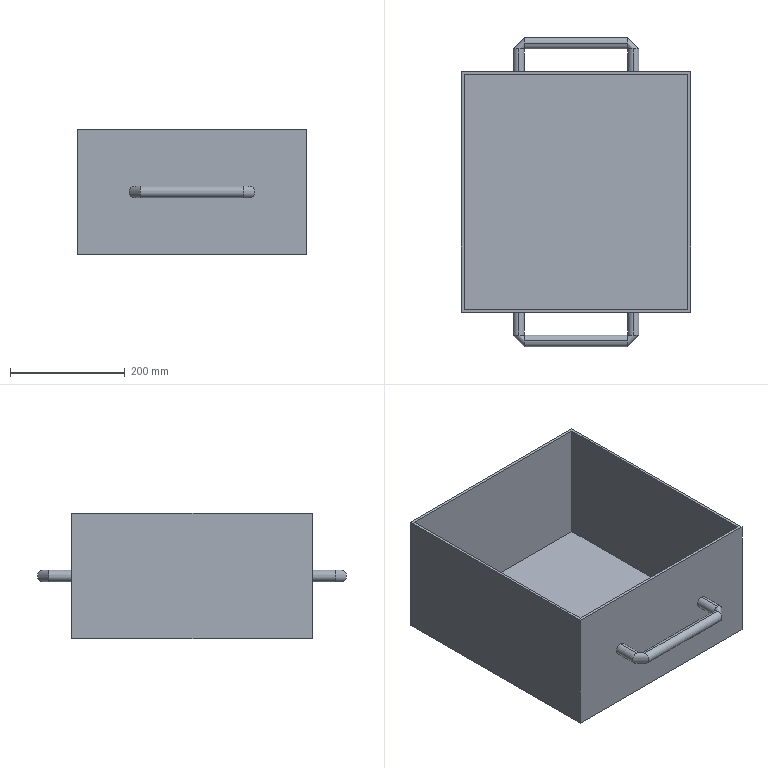Part | STEP file | Scrap collection box | 1 solid | 27 faces | box 400 x 540 x 220 mm | volume 2744863 mm3 | cylinder 12 | plane 11 | torus 4 | commonest cylinder face diameters 20 x12
STEP:
#1=CARTESIAN_POINT('',(100.,250.,-10.));
#2=VERTEX_POINT('',#1);
#3=CARTESIAN_POINT('',(100.,250.,10.));
#4=VERTEX_POINT('',#3);
#5=CARTESIAN_POINT('',(100.,250.,0.));
#6=DIRECTION('',(0.,-1.,0.));
#7=DIRECTION('',(0.,0.,-1.));
#8=AXIS2_PLACEMENT_3D('',#5,#6,#7);
#9=CIRCLE('',#8,10.);
#10=EDGE_CURVE('',#2,#4,#9,.T.);
#11=ORIENTED_EDGE('',*,*,#10,.T.);
#12=CARTESIAN_POINT('',(100.,210.,10.));
#13=VERTEX_POINT('',#12);
#14=CARTESIAN_POINT('',(100.,250.,10.));
#15=DIRECTION('',(0.,-1.,0.));
#16=VECTOR('',#15,1000.);
#17=LINE('',#14,#16);
#18=EDGE_CURVE('',#4,#13,#17,.T.);
#19=ORIENTED_EDGE('',*,*,#18,.T.);
#20=CARTESIAN_POINT('',(100.,210.,-10.));
#21=VERTEX_POINT('',#20);
#22=CARTESIAN_POINT('',(100.,210.,0.));
#23=DIRECTION('',(0.,-1.,0.));
#24=DIRECTION('',(0.,0.,-1.));
#25=AXIS2_PLACEMENT_3D('',#22,#23,#24);
#26=CIRCLE('',#25,10.);
#27=EDGE_CURVE('',#21,#13,#26,.T.);
#28=ORIENTED_EDGE('',*,*,#27,.F.);
#29=CARTESIAN_POINT('',(100.,250.,-10.));
#30=DIRECTION('',(0.,-1.,0.));
#31=VECTOR('',#30,1000.);
#32=LINE('',#29,#31);
#33=EDGE_CURVE('',#2,#21,#32,.T.);
#34=ORIENTED_EDGE('',*,*,#33,.F.);
#35=EDGE_LOOP('',(#11,#19,#28,#34));
#36=FACE_OUTER_BOUND('',#35,.T.);
#37=CARTESIAN_POINT('',(100.,250.,0.));
#38=DIRECTION('',(0.,-1.,0.));
#39=DIRECTION('',(0.,0.,-1.));
#40=AXIS2_PLACEMENT_3D('',#37,#38,#39);
#41=CYLINDRICAL_SURFACE('',#40,10.);
#42=ADVANCED_FACE('',(#36),#41,.T.);
#43=CARTESIAN_POINT('',(-90.,260.,-10.));
#44=VERTEX_POINT('',#43);
#45=CARTESIAN_POINT('',(-90.,260.,10.));
#46=VERTEX_POINT('',#45);
#47=CARTESIAN_POINT('',(-90.,260.,0.));
#48=DIRECTION('',(1.,0.,0.));
#49=DIRECTION('',(0.,0.,-1.));
#50=AXIS2_PLACEMENT_3D('',#47,#48,#49);
#51=CIRCLE('',#50,10.);
#52=EDGE_CURVE('',#44,#46,#51,.T.);
#53=ORIENTED_EDGE('',*,*,#52,.T.);
#54=CARTESIAN_POINT('',(90.,260.,10.));
#55=VERTEX_POINT('',#54);
#56=CARTESIAN_POINT('',(-90.,260.,10.));
#57=DIRECTION('',(1.,0.,0.));
#58=VECTOR('',#57,1000.);
#59=LINE('',#56,#58);
#60=EDGE_CURVE('',#46,#55,#59,.T.);
#61=ORIENTED_EDGE('',*,*,#60,.T.);
#62=CARTESIAN_POINT('',(90.,260.,-10.));
#63=VERTEX_POINT('',#62);
#64=CARTESIAN_POINT('',(90.,260.,0.));
#65=DIRECTION('',(1.,0.,0.));
#66=DIRECTION('',(0.,0.,-1.));
#67=AXIS2_PLACEMENT_3D('',#64,#65,#66);
#68=CIRCLE('',#67,10.);
#69=EDGE_CURVE('',#63,#55,#68,.T.);
#70=ORIENTED_EDGE('',*,*,#69,.F.);
#71=CARTESIAN_POINT('',(-90.,260.,-10.));
#72=DIRECTION('',(1.,0.,0.));
#73=VECTOR('',#72,1000.);
#74=LINE('',#71,#73);
#75=EDGE_CURVE('',#44,#63,#74,.T.);
#76=ORIENTED_EDGE('',*,*,#75,.F.);
#77=EDGE_LOOP('',(#53,#61,#70,#76));
#78=FACE_OUTER_BOUND('',#77,.T.);
#79=CARTESIAN_POINT('',(-90.,260.,0.));
#80=DIRECTION('',(1.,0.,0.));
#81=DIRECTION('',(0.,0.,-1.));
#82=AXIS2_PLACEMENT_3D('',#79,#80,#81);
#83=CYLINDRICAL_SURFACE('',#82,10.);
#84=ADVANCED_FACE('',(#78),#83,.T.);
#85=CARTESIAN_POINT('',(-100.,210.,10.));
#86=VERTEX_POINT('',#85);
#87=CARTESIAN_POINT('',(-100.,210.,-10.));
#88=VERTEX_POINT('',#87);
#89=CARTESIAN_POINT('',(-100.,210.,0.));
#90=DIRECTION('',(0.,1.,0.));
#91=DIRECTION('',(0.,0.,-1.));
#92=AXIS2_PLACEMENT_3D('',#89,#90,#91);
#93=CIRCLE('',#92,10.);
#94=EDGE_CURVE('',#86,#88,#93,.T.);
#95=ORIENTED_EDGE('',*,*,#94,.T.);
#96=CARTESIAN_POINT('',(-100.,250.,-10.));
#97=VERTEX_POINT('',#96);
#98=CARTESIAN_POINT('',(-100.,210.,-10.));
#99=DIRECTION('',(0.,1.,0.));
#100=VECTOR('',#99,1000.);
#101=LINE('',#98,#100);
#102=EDGE_CURVE('',#88,#97,#101,.T.);
#103=ORIENTED_EDGE('',*,*,#102,.T.);
#104=CARTESIAN_POINT('',(-90.,250.,0.));
#105=VERTEX_POINT('',#104);
#106=CARTESIAN_POINT('',(-100.,250.,0.));
#107=DIRECTION('',(0.,1.,0.));
#108=DIRECTION('',(0.,0.,-1.));
#109=AXIS2_PLACEMENT_3D('',#106,#107,#108);
#110=CIRCLE('',#109,10.);
#111=EDGE_CURVE('',#105,#97,#110,.T.);
#112=ORIENTED_EDGE('',*,*,#111,.F.);
#113=CARTESIAN_POINT('',(-100.,250.,10.));
#114=VERTEX_POINT('',#113);
#115=CARTESIAN_POINT('',(-100.,250.,0.));
#116=DIRECTION('',(0.,1.,0.));
#117=DIRECTION('',(0.,0.,-1.));
#118=AXIS2_PLACEMENT_3D('',#115,#116,#117);
#119=CIRCLE('',#118,10.);
#120=EDGE_CURVE('',#114,#105,#119,.T.);
#121=ORIENTED_EDGE('',*,*,#120,.F.);
#122=CARTESIAN_POINT('',(-100.,210.,10.));
#123=DIRECTION('',(0.,1.,0.));
#124=VECTOR('',#123,1000.);
#125=LINE('',#122,#124);
#126=EDGE_CURVE('',#86,#114,#125,.T.);
#127=ORIENTED_EDGE('',*,*,#126,.F.);
#128=EDGE_LOOP('',(#95,#103,#112,#121,#127));
#129=FACE_OUTER_BOUND('',#128,.T.);
#130=CARTESIAN_POINT('',(-100.,210.,0.));
#131=DIRECTION('',(0.,1.,0.));
#132=DIRECTION('',(0.,0.,1.));
#133=AXIS2_PLACEMENT_3D('',#130,#131,#132);
#134=CYLINDRICAL_SURFACE('',#133,10.);
#135=ADVANCED_FACE('',(#129),#134,.T.);
#136=CARTESIAN_POINT('',(100.,-250.,10.));
#137=VERTEX_POINT('',#136);
#138=CARTESIAN_POINT('',(100.,-250.,-10.));
#139=VERTEX_POINT('',#138);
#140=CARTESIAN_POINT('',(100.,-250.,0.));
#141=DIRECTION('',(0.,1.,0.));
#142=DIRECTION('',(0.,0.,-1.));
#143=AXIS2_PLACEMENT_3D('',#140,#141,#142);
#144=CIRCLE('',#143,10.);
#145=EDGE_CURVE('',#137,#139,#144,.T.);
#146=ORIENTED_EDGE('',*,*,#145,.T.);
#147=CARTESIAN_POINT('',(100.,-210.,-10.));
#148=VERTEX_POINT('',#147);
#149=CARTESIAN_POINT('',(100.,-250.,-10.));
#150=DIRECTION('',(0.,1.,0.));
#151=VECTOR('',#150,1000.);
#152=LINE('',#149,#151);
#153=EDGE_CURVE('',#139,#148,#152,.T.);
#154=ORIENTED_EDGE('',*,*,#153,.T.);
#155=CARTESIAN_POINT('',(100.,-210.,10.));
#156=VERTEX_POINT('',#155);
#157=CARTESIAN_POINT('',(100.,-210.,0.));
#158=DIRECTION('',(0.,1.,0.));
#159=DIRECTION('',(0.,0.,-1.));
#160=AXIS2_PLACEMENT_3D('',#157,#158,#159);
#161=CIRCLE('',#160,10.);
#162=EDGE_CURVE('',#156,#148,#161,.T.);
#163=ORIENTED_EDGE('',*,*,#162,.F.);
#164=CARTESIAN_POINT('',(100.,-250.,10.));
#165=DIRECTION('',(0.,1.,0.));
#166=VECTOR('',#165,1000.);
#167=LINE('',#164,#166);
#168=EDGE_CURVE('',#137,#156,#167,.T.);
#169=ORIENTED_EDGE('',*,*,#168,.F.);
#170=EDGE_LOOP('',(#146,#154,#163,#169));
#171=FACE_OUTER_BOUND('',#170,.T.);
#172=CARTESIAN_POINT('',(100.,-250.,0.));
#173=DIRECTION('',(0.,1.,0.));
#174=DIRECTION('',(0.,0.,1.));
#175=AXIS2_PLACEMENT_3D('',#172,#173,#174);
#176=CYLINDRICAL_SURFACE('',#175,10.);
#177=ADVANCED_FACE('',(#171),#176,.T.);
#178=CARTESIAN_POINT('',(-90.,-250.,0.));
#179=VERTEX_POINT('',#178);
#180=CARTESIAN_POINT('',(-90.,-260.,10.));
#181=VERTEX_POINT('',#180);
#182=CARTESIAN_POINT('',(-90.,-260.,0.));
#183=DIRECTION('',(1.,0.,0.));
#184=DIRECTION('',(0.,0.,-1.));
#185=AXIS2_PLACEMENT_3D('',#182,#183,#184);
#186=CIRCLE('',#185,10.);
#187=EDGE_CURVE('',#179,#181,#186,.T.);
#188=ORIENTED_EDGE('',*,*,#187,.T.);
#189=CARTESIAN_POINT('',(90.,-260.,10.));
#190=VERTEX_POINT('',#189);
#191=CARTESIAN_POINT('',(-90.,-260.,10.));
#192=DIRECTION('',(1.,0.,0.));
#193=VECTOR('',#192,1000.);
#194=LINE('',#191,#193);
#195=EDGE_CURVE('',#181,#190,#194,.T.);
#196=ORIENTED_EDGE('',*,*,#195,.T.);
#197=CARTESIAN_POINT('',(90.,-250.,0.));
#198=VERTEX_POINT('',#197);
#199=CARTESIAN_POINT('',(90.,-260.,0.));
#200=DIRECTION('',(1.,0.,0.));
#201=DIRECTION('',(0.,0.,-1.));
#202=AXIS2_PLACEMENT_3D('',#199,#200,#201);
#203=CIRCLE('',#202,10.);
#204=EDGE_CURVE('',#198,#190,#203,.T.);
#205=ORIENTED_EDGE('',*,*,#204,.F.);
#206=CARTESIAN_POINT('',(90.,-260.,-10.));
#207=VERTEX_POINT('',#206);
#208=CARTESIAN_POINT('',(90.,-260.,0.));
#209=DIRECTION('',(1.,0.,0.));
#210=DIRECTION('',(0.,0.,-1.));
#211=AXIS2_PLACEMENT_3D('',#208,#209,#210);
#212=CIRCLE('',#211,10.);
#213=EDGE_CURVE('',#207,#198,#212,.T.);
#214=ORIENTED_EDGE('',*,*,#213,.F.);
#215=CARTESIAN_POINT('',(-90.,-260.,-10.));
#216=VERTEX_POINT('',#215);
#217=CARTESIAN_POINT('',(-90.,-260.,-10.));
#218=DIRECTION('',(1.,0.,0.));
#219=VECTOR('',#218,1000.);
#220=LINE('',#217,#219);
#221=EDGE_CURVE('',#216,#207,#220,.T.);
#222=ORIENTED_EDGE('',*,*,#221,.F.);
#223=CARTESIAN_POINT('',(-90.,-260.,0.));
#224=DIRECTION('',(1.,0.,0.));
#225=DIRECTION('',(0.,0.,-1.));
#226=AXIS2_PLACEMENT_3D('',#223,#224,#225);
#227=CIRCLE('',#226,10.);
#228=EDGE_CURVE('',#216,#179,#227,.T.);
#229=ORIENTED_EDGE('',*,*,#228,.T.);
#230=EDGE_LOOP('',(#188,#196,#205,#214,#222,#229));
#231=FACE_OUTER_BOUND('',#230,.T.);
#232=CARTESIAN_POINT('',(-90.,-260.,0.));
#233=DIRECTION('',(1.,0.,0.));
#234=DIRECTION('',(0.,0.,-1.));
#235=AXIS2_PLACEMENT_3D('',#232,#233,#234);
#236=CYLINDRICAL_SURFACE('',#235,10.);
#237=ADVANCED_FACE('',(#231),#236,.T.);
#238=CARTESIAN_POINT('',(-100.,-210.,-10.));
#239=VERTEX_POINT('',#238);
#240=CARTESIAN_POINT('',(-100.,-210.,10.));
#241=VERTEX_POINT('',#240);
#242=CARTESIAN_POINT('',(-100.,-210.,0.));
#243=DIRECTION('',(0.,-1.,0.));
#244=DIRECTION('',(0.,0.,-1.));
#245=AXIS2_PLACEMENT_3D('',#242,#243,#244);
#246=CIRCLE('',#245,10.);
#247=EDGE_CURVE('',#239,#241,#246,.T.);
#248=ORIENTED_EDGE('',*,*,#247,.T.);
#249=CARTESIAN_POINT('',(-100.,-250.,10.));
#250=VERTEX_POINT('',#249);
#251=CARTESIAN_POINT('',(-100.,-210.,10.));
#252=DIRECTION('',(0.,-1.,0.));
#253=VECTOR('',#252,1000.);
#254=LINE('',#251,#253);
#255=EDGE_CURVE('',#241,#250,#254,.T.);
#256=ORIENTED_EDGE('',*,*,#255,.T.);
#257=CARTESIAN_POINT('',(-100.,-250.,0.));
#258=DIRECTION('',(0.,-1.,0.));
#259=DIRECTION('',(0.,0.,-1.));
#260=AXIS2_PLACEMENT_3D('',#257,#258,#259);
#261=CIRCLE('',#260,10.);
#262=EDGE_CURVE('',#179,#250,#261,.T.);
#263=ORIENTED_EDGE('',*,*,#262,.F.);
#264=CARTESIAN_POINT('',(-100.,-250.,-10.));
#265=VERTEX_POINT('',#264);
#266=CARTESIAN_POINT('',(-100.,-250.,0.));
#267=DIRECTION('',(0.,-1.,0.));
#268=DIRECTION('',(0.,0.,-1.));
#269=AXIS2_PLACEMENT_3D('',#266,#267,#268);
#270=CIRCLE('',#269,10.);
#271=EDGE_CURVE('',#265,#179,#270,.T.);
#272=ORIENTED_EDGE('',*,*,#271,.F.);
#273=CARTESIAN_POINT('',(-100.,-210.,-10.));
#274=DIRECTION('',(0.,-1.,0.));
#275=VECTOR('',#274,1000.);
#276=LINE('',#273,#275);
#277=EDGE_CURVE('',#239,#265,#276,.T.);
#278=ORIENTED_EDGE('',*,*,#277,.F.);
#279=EDGE_LOOP('',(#248,#256,#263,#272,#278));
#280=FACE_OUTER_BOUND('',#279,.T.);
#281=CARTESIAN_POINT('',(-100.,-210.,0.));
#282=DIRECTION('',(0.,-1.,0.));
#283=DIRECTION('',(0.,0.,-1.));
#284=AXIS2_PLACEMENT_3D('',#281,#282,#283);
#285=CYLINDRICAL_SURFACE('',#284,10.);
#286=ADVANCED_FACE('',(#280),#285,.T.);
#287=CARTESIAN_POINT('',(200.,-210.,-110.));
#288=VERTEX_POINT('',#287);
#289=CARTESIAN_POINT('',(200.,210.,-110.));
#290=VERTEX_POINT('',#289);
#291=CARTESIAN_POINT('',(200.,210.,-110.));
#292=DIRECTION('',(0.,1.,0.));
#293=VECTOR('',#292,1000.);
#294=LINE('',#291,#293);
#295=EDGE_CURVE('',#288,#290,#294,.T.);
#296=ORIENTED_EDGE('',*,*,#295,.T.);
#297=CARTESIAN_POINT('',(200.,210.,110.));
#298=VERTEX_POINT('',#297);
#299=CARTESIAN_POINT('',(200.,210.,110.));
#300=DIRECTION('',(0.,0.,-1.));
#301=VECTOR('',#300,1000.);
#302=LINE('',#299,#301);
#303=EDGE_CURVE('',#298,#290,#302,.T.);
#304=ORIENTED_EDGE('',*,*,#303,.F.);
#305=CARTESIAN_POINT('',(200.,-210.,110.));
#306=VERTEX_POINT('',#305);
#307=CARTESIAN_POINT('',(200.,210.,110.));
#308=DIRECTION('',(0.,1.,0.));
#309=VECTOR('',#308,1000.);
#310=LINE('',#307,#309);
#311=EDGE_CURVE('',#306,#298,#310,.T.);
#312=ORIENTED_EDGE('',*,*,#311,.F.);
#313=CARTESIAN_POINT('',(200.,-210.,110.));
#314=DIRECTION('',(0.,0.,-1.));
#315=VECTOR('',#314,1000.);
#316=LINE('',#313,#315);
#317=EDGE_CURVE('',#306,#288,#316,.T.);
#318=ORIENTED_EDGE('',*,*,#317,.T.);
#319=EDGE_LOOP('',(#296,#304,#312,#318));
#320=FACE_OUTER_BOUND('',#319,.T.);
#321=CARTESIAN_POINT('',(200.,210.,110.));
#322=DIRECTION('',(-1.,0.,0.));
#323=DIRECTION('',(0.,-1.,0.));
#324=AXIS2_PLACEMENT_3D('',#321,#322,#323);
#325=PLANE('',#324);
#326=ADVANCED_FACE('',(#320),#325,.F.);
#327=ORIENTED_EDGE('',*,*,#94,.F.);
#328=CARTESIAN_POINT('',(-100.,210.,0.));
#329=DIRECTION('',(0.,1.,0.));
#330=DIRECTION('',(0.,0.,-1.));
#331=AXIS2_PLACEMENT_3D('',#328,#329,#330);
#332=CIRCLE('',#331,10.);
#333=EDGE_CURVE('',#88,#86,#332,.T.);
#334=ORIENTED_EDGE('',*,*,#333,.F.);
#335=EDGE_LOOP('',(#327,#334));
#336=FACE_BOUND('',#335,.T.);
#337=ORIENTED_EDGE('',*,*,#27,.T.);
#338=CARTESIAN_POINT('',(100.,210.,0.));
#339=DIRECTION('',(0.,-1.,0.));
#340=DIRECTION('',(0.,0.,-1.));
#341=AXIS2_PLACEMENT_3D('',#338,#339,#340);
#342=CIRCLE('',#341,10.);
#343=EDGE_CURVE('',#13,#21,#342,.T.);
#344=ORIENTED_EDGE('',*,*,#343,.T.);
#345=EDGE_LOOP('',(#337,#344));
#346=FACE_BOUND('',#345,.T.);
#347=CARTESIAN_POINT('',(-200.,210.,-110.));
#348=VERTEX_POINT('',#347);
#349=CARTESIAN_POINT('',(-200.,210.,-110.));
#350=DIRECTION('',(-1.,0.,0.));
#351=VECTOR('',#350,1000.);
#352=LINE('',#349,#351);
#353=EDGE_CURVE('',#290,#348,#352,.T.);
#354=ORIENTED_EDGE('',*,*,#353,.T.);
#355=CARTESIAN_POINT('',(-200.,210.,110.));
#356=VERTEX_POINT('',#355);
#357=CARTESIAN_POINT('',(-200.,210.,110.));
#358=DIRECTION('',(0.,0.,-1.));
#359=VECTOR('',#358,1000.);
#360=LINE('',#357,#359);
#361=EDGE_CURVE('',#356,#348,#360,.T.);
#362=ORIENTED_EDGE('',*,*,#361,.F.);
#363=CARTESIAN_POINT('',(-200.,210.,110.));
#364=DIRECTION('',(-1.,0.,0.));
#365=VECTOR('',#364,1000.);
#366=LINE('',#363,#365);
#367=EDGE_CURVE('',#298,#356,#366,.T.);
#368=ORIENTED_EDGE('',*,*,#367,.F.);
#369=ORIENTED_EDGE('',*,*,#303,.T.);
#370=EDGE_LOOP('',(#354,#362,#368,#369));
#371=FACE_OUTER_BOUND('',#370,.T.);
#372=CARTESIAN_POINT('',(-200.,210.,110.));
#373=DIRECTION('',(0.,-1.,0.));
#374=DIRECTION('',(0.,0.,-1.));
#375=AXIS2_PLACEMENT_3D('',#372,#373,#374);
#376=PLANE('',#375);
#377=ADVANCED_FACE('',(#336,#346,#371),#376,.F.);
#378=CARTESIAN_POINT('',(-200.,-210.,-110.));
#379=VERTEX_POINT('',#378);
#380=CARTESIAN_POINT('',(-200.,210.,-110.));
#381=DIRECTION('',(0.,-1.,0.));
#382=VECTOR('',#381,1000.);
#383=LINE('',#380,#382);
#384=EDGE_CURVE('',#348,#379,#383,.T.);
#385=ORIENTED_EDGE('',*,*,#384,.T.);
#386=CARTESIAN_POINT('',(-200.,-210.,110.));
#387=VERTEX_POINT('',#386);
#388=CARTESIAN_POINT('',(-200.,-210.,110.));
#389=DIRECTION('',(0.,0.,-1.));
#390=VECTOR('',#389,1000.);
#391=LINE('',#388,#390);
#392=EDGE_CURVE('',#387,#379,#391,.T.);
#393=ORIENTED_EDGE('',*,*,#392,.F.);
#394=CARTESIAN_POINT('',(-200.,210.,110.));
#395=DIRECTION('',(0.,-1.,0.));
#396=VECTOR('',#395,1000.);
#397=LINE('',#394,#396);
#398=EDGE_CURVE('',#356,#387,#397,.T.);
#399=ORIENTED_EDGE('',*,*,#398,.F.);
#400=ORIENTED_EDGE('',*,*,#361,.T.);
#401=EDGE_LOOP('',(#385,#393,#399,#400));
#402=FACE_OUTER_BOUND('',#401,.T.);
#403=CARTESIAN_POINT('',(-200.,210.,110.));
#404=DIRECTION('',(1.,0.,0.));
#405=DIRECTION('',(0.,1.,0.));
#406=AXIS2_PLACEMENT_3D('',#403,#404,#405);
#407=PLANE('',#406);
#408=ADVANCED_FACE('',(#402),#407,.F.);
#409=ORIENTED_EDGE('',*,*,#247,.F.);
#410=CARTESIAN_POINT('',(-100.,-210.,0.));
#411=DIRECTION('',(0.,-1.,0.));
#412=DIRECTION('',(0.,0.,-1.));
#413=AXIS2_PLACEMENT_3D('',#410,#411,#412);
#414=CIRCLE('',#413,10.);
#415=EDGE_CURVE('',#241,#239,#414,.T.);
#416=ORIENTED_EDGE('',*,*,#415,.F.);
#417=EDGE_LOOP('',(#409,#416));
#418=FACE_BOUND('',#417,.T.);
#419=ORIENTED_EDGE('',*,*,#162,.T.);
#420=CARTESIAN_POINT('',(100.,-210.,0.));
#421=DIRECTION('',(0.,1.,0.));
#422=DIRECTION('',(0.,0.,-1.));
#423=AXIS2_PLACEMENT_3D('',#420,#421,#422);
#424=CIRCLE('',#423,10.);
#425=EDGE_CURVE('',#148,#156,#424,.T.);
#426=ORIENTED_EDGE('',*,*,#425,.T.);
#427=EDGE_LOOP('',(#419,#426));
#428=FACE_BOUND('',#427,.T.);
#429=CARTESIAN_POINT('',(-200.,-210.,-110.));
#430=DIRECTION('',(1.,0.,0.));
#431=VECTOR('',#430,1000.);
#432=LINE('',#429,#431);
#433=EDGE_CURVE('',#379,#288,#432,.T.);
#434=ORIENTED_EDGE('',*,*,#433,.T.);
#435=ORIENTED_EDGE('',*,*,#317,.F.);
#436=CARTESIAN_POINT('',(-200.,-210.,110.));
#437=DIRECTION('',(1.,0.,0.));
#438=VECTOR('',#437,1000.);
#439=LINE('',#436,#438);
#440=EDGE_CURVE('',#387,#306,#439,.T.);
#441=ORIENTED_EDGE('',*,*,#440,.F.);
#442=ORIENTED_EDGE('',*,*,#392,.T.);
#443=EDGE_LOOP('',(#434,#435,#441,#442));
#444=FACE_OUTER_BOUND('',#443,.T.);
#445=CARTESIAN_POINT('',(-200.,-210.,110.));
#446=DIRECTION('',(0.,1.,0.));
#447=DIRECTION('',(0.,0.,1.));
#448=AXIS2_PLACEMENT_3D('',#445,#446,#447);
#449=PLANE('',#448);
#450=ADVANCED_FACE('',(#418,#428,#444),#449,.F.);
#451=CARTESIAN_POINT('',(195.,-205.,110.));
#452=VERTEX_POINT('',#451);
#453=CARTESIAN_POINT('',(195.,205.,110.));
#454=VERTEX_POINT('',#453);
#455=CARTESIAN_POINT('',(195.,210.,110.));
#456=DIRECTION('',(0.,1.,0.));
#457=VECTOR('',#456,1000.);
#458=LINE('',#455,#457);
#459=EDGE_CURVE('',#452,#454,#458,.T.);
#460=ORIENTED_EDGE('',*,*,#459,.F.);
#461=CARTESIAN_POINT('',(-195.,-205.,110.));
#462=VERTEX_POINT('',#461);
#463=CARTESIAN_POINT('',(-200.,-205.,110.));
#464=DIRECTION('',(1.,0.,0.));
#465=VECTOR('',#464,1000.);
#466=LINE('',#463,#465);
#467=EDGE_CURVE('',#462,#452,#466,.T.);
#468=ORIENTED_EDGE('',*,*,#467,.F.);
#469=CARTESIAN_POINT('',(-195.,205.,110.));
#470=VERTEX_POINT('',#469);
#471=CARTESIAN_POINT('',(-195.,210.,110.));
#472=DIRECTION('',(0.,-1.,0.));
#473=VECTOR('',#472,1000.);
#474=LINE('',#471,#473);
#475=EDGE_CURVE('',#470,#462,#474,.T.);
#476=ORIENTED_EDGE('',*,*,#475,.F.);
#477=CARTESIAN_POINT('',(-200.,205.,110.));
#478=DIRECTION('',(-1.,0.,0.));
#479=VECTOR('',#478,1000.);
#480=LINE('',#477,#479);
#481=EDGE_CURVE('',#454,#470,#480,.T.);
#482=ORIENTED_EDGE('',*,*,#481,.F.);
#483=EDGE_LOOP('',(#460,#468,#476,#482));
#484=FACE_BOUND('',#483,.T.);
#485=ORIENTED_EDGE('',*,*,#311,.T.);
#486=ORIENTED_EDGE('',*,*,#367,.T.);
#487=ORIENTED_EDGE('',*,*,#398,.T.);
#488=ORIENTED_EDGE('',*,*,#440,.T.);
#489=EDGE_LOOP('',(#485,#486,#487,#488));
#490=FACE_OUTER_BOUND('',#489,.T.);
#491=CARTESIAN_POINT('',(0.,0.,110.));
#492=DIRECTION('',(0.,0.,1.));
#493=DIRECTION('',(1.,0.,0.));
#494=AXIS2_PLACEMENT_3D('',#491,#492,#493);
#495=PLANE('',#494);
#496=ADVANCED_FACE('',(#484,#490),#495,.T.);
#497=ORIENTED_EDGE('',*,*,#295,.F.);
#498=ORIENTED_EDGE('',*,*,#433,.F.);
#499=ORIENTED_EDGE('',*,*,#384,.F.);
#500=ORIENTED_EDGE('',*,*,#353,.F.);
#501=EDGE_LOOP('',(#497,#498,#499,#500));
#502=FACE_OUTER_BOUND('',#501,.T.);
#503=CARTESIAN_POINT('',(0.,0.,-110.));
#504=DIRECTION('',(0.,0.,1.));
#505=DIRECTION('',(1.,0.,0.));
#506=AXIS2_PLACEMENT_3D('',#503,#504,#505);
#507=PLANE('',#506);
#508=ADVANCED_FACE('',(#502),#507,.F.);
#509=CARTESIAN_POINT('',(195.,-205.,-105.));
#510=VERTEX_POINT('',#509);
#511=CARTESIAN_POINT('',(195.,205.,-105.));
#512=VERTEX_POINT('',#511);
#513=CARTESIAN_POINT('',(195.,210.,-105.));
#514=DIRECTION('',(0.,1.,0.));
#515=VECTOR('',#514,1000.);
#516=LINE('',#513,#515);
#517=EDGE_CURVE('',#510,#512,#516,.T.);
#518=ORIENTED_EDGE('',*,*,#517,.F.);
#519=CARTESIAN_POINT('',(195.,-205.,110.));
#520=DIRECTION('',(0.,0.,-1.));
#521=VECTOR('',#520,1000.);
#522=LINE('',#519,#521);
#523=EDGE_CURVE('',#452,#510,#522,.T.);
#524=ORIENTED_EDGE('',*,*,#523,.F.);
#525=ORIENTED_EDGE('',*,*,#459,.T.);
#526=CARTESIAN_POINT('',(195.,205.,110.));
#527=DIRECTION('',(0.,0.,-1.));
#528=VECTOR('',#527,1000.);
#529=LINE('',#526,#528);
#530=EDGE_CURVE('',#454,#512,#529,.T.);
#531=ORIENTED_EDGE('',*,*,#530,.T.);
#532=EDGE_LOOP('',(#518,#524,#525,#531));
#533=FACE_OUTER_BOUND('',#532,.T.);
#534=CARTESIAN_POINT('',(195.,210.,110.));
#535=DIRECTION('',(-1.,0.,0.));
#536=DIRECTION('',(0.,-1.,0.));
#537=AXIS2_PLACEMENT_3D('',#534,#535,#536);
#538=PLANE('',#537);
#539=ADVANCED_FACE('',(#533),#538,.T.);
#540=CARTESIAN_POINT('',(-195.,205.,-105.));
#541=VERTEX_POINT('',#540);
#542=CARTESIAN_POINT('',(-200.,205.,-105.));
#543=DIRECTION('',(-1.,0.,0.));
#544=VECTOR('',#543,1000.);
#545=LINE('',#542,#544);
#546=EDGE_CURVE('',#512,#541,#545,.T.);
#547=ORIENTED_EDGE('',*,*,#546,.F.);
#548=ORIENTED_EDGE('',*,*,#530,.F.);
#549=ORIENTED_EDGE('',*,*,#481,.T.);
#550=CARTESIAN_POINT('',(-195.,205.,110.));
#551=DIRECTION('',(0.,0.,-1.));
#552=VECTOR('',#551,1000.);
#553=LINE('',#550,#552);
#554=EDGE_CURVE('',#470,#541,#553,.T.);
#555=ORIENTED_EDGE('',*,*,#554,.T.);
#556=EDGE_LOOP('',(#547,#548,#549,#555));
#557=FACE_OUTER_BOUND('',#556,.T.);
#558=CARTESIAN_POINT('',(-200.,205.,110.));
#559=DIRECTION('',(0.,-1.,0.));
#560=DIRECTION('',(0.,0.,-1.));
#561=AXIS2_PLACEMENT_3D('',#558,#559,#560);
#562=PLANE('',#561);
#563=ADVANCED_FACE('',(#557),#562,.T.);
#564=CARTESIAN_POINT('',(-195.,-205.,-105.));
#565=VERTEX_POINT('',#564);
#566=CARTESIAN_POINT('',(-195.,210.,-105.));
#567=DIRECTION('',(0.,-1.,0.));
#568=VECTOR('',#567,1000.);
#569=LINE('',#566,#568);
#570=EDGE_CURVE('',#541,#565,#569,.T.);
#571=ORIENTED_EDGE('',*,*,#570,.F.);
#572=ORIENTED_EDGE('',*,*,#554,.F.);
#573=ORIENTED_EDGE('',*,*,#475,.T.);
#574=CARTESIAN_POINT('',(-195.,-205.,110.));
#575=DIRECTION('',(0.,0.,-1.));
#576=VECTOR('',#575,1000.);
#577=LINE('',#574,#576);
#578=EDGE_CURVE('',#462,#565,#577,.T.);
#579=ORIENTED_EDGE('',*,*,#578,.T.);
#580=EDGE_LOOP('',(#571,#572,#573,#579));
#581=FACE_OUTER_BOUND('',#580,.T.);
#582=CARTESIAN_POINT('',(-195.,210.,110.));
#583=DIRECTION('',(1.,0.,0.));
#584=DIRECTION('',(0.,1.,0.));
#585=AXIS2_PLACEMENT_3D('',#582,#583,#584);
#586=PLANE('',#585);
#587=ADVANCED_FACE('',(#581),#586,.T.);
#588=CARTESIAN_POINT('',(-200.,-205.,-105.));
#589=DIRECTION('',(1.,0.,0.));
#590=VECTOR('',#589,1000.);
#591=LINE('',#588,#590);
#592=EDGE_CURVE('',#565,#510,#591,.T.);
#593=ORIENTED_EDGE('',*,*,#592,.F.);
#594=ORIENTED_EDGE('',*,*,#578,.F.);
#595=ORIENTED_EDGE('',*,*,#467,.T.);
#596=ORIENTED_EDGE('',*,*,#523,.T.);
#597=EDGE_LOOP('',(#593,#594,#595,#596));
#598=FACE_OUTER_BOUND('',#597,.T.);
#599=CARTESIAN_POINT('',(-200.,-205.,110.));
#600=DIRECTION('',(0.,1.,0.));
#601=DIRECTION('',(0.,0.,1.));
#602=AXIS2_PLACEMENT_3D('',#599,#600,#601);
#603=PLANE('',#602);
#604=ADVANCED_FACE('',(#598),#603,.T.);
#605=ORIENTED_EDGE('',*,*,#517,.T.);
#606=ORIENTED_EDGE('',*,*,#546,.T.);
#607=ORIENTED_EDGE('',*,*,#570,.T.);
#608=ORIENTED_EDGE('',*,*,#592,.T.);
#609=EDGE_LOOP('',(#605,#606,#607,#608));
#610=FACE_OUTER_BOUND('',#609,.T.);
#611=CARTESIAN_POINT('',(0.,0.,-105.));
#612=DIRECTION('',(0.,0.,1.));
#613=DIRECTION('',(1.,0.,0.));
#614=AXIS2_PLACEMENT_3D('',#611,#612,#613);
#615=PLANE('',#614);
#616=ADVANCED_FACE('',(#610),#615,.T.);
#617=ORIENTED_EDGE('',*,*,#153,.F.);
#618=CARTESIAN_POINT('',(100.,-250.,0.));
#619=DIRECTION('',(0.,1.,0.));
#620=DIRECTION('',(0.,0.,-1.));
#621=AXIS2_PLACEMENT_3D('',#618,#619,#620);
#622=CIRCLE('',#621,10.);
#623=EDGE_CURVE('',#139,#198,#622,.T.);
#624=ORIENTED_EDGE('',*,*,#623,.T.);
#625=CARTESIAN_POINT('',(100.,-250.,0.));
#626=DIRECTION('',(0.,1.,0.));
#627=DIRECTION('',(0.,0.,-1.));
#628=AXIS2_PLACEMENT_3D('',#625,#626,#627);
#629=CIRCLE('',#628,10.);
#630=EDGE_CURVE('',#198,#137,#629,.T.);
#631=ORIENTED_EDGE('',*,*,#630,.T.);
#632=ORIENTED_EDGE('',*,*,#168,.T.);
#633=ORIENTED_EDGE('',*,*,#425,.F.);
#634=EDGE_LOOP('',(#617,#624,#631,#632,#633));
#635=FACE_OUTER_BOUND('',#634,.T.);
#636=CARTESIAN_POINT('',(100.,-250.,0.));
#637=DIRECTION('',(0.,1.,0.));
#638=DIRECTION('',(0.,0.,1.));
#639=AXIS2_PLACEMENT_3D('',#636,#637,#638);
#640=CYLINDRICAL_SURFACE('',#639,10.);
#641=ADVANCED_FACE('',(#635),#640,.T.);
#642=ORIENTED_EDGE('',*,*,#630,.F.);
#643=ORIENTED_EDGE('',*,*,#204,.T.);
#644=CARTESIAN_POINT('',(90.,-260.,0.));
#645=DIRECTION('',(1.,0.,0.));
#646=DIRECTION('',(0.,0.,-1.));
#647=AXIS2_PLACEMENT_3D('',#644,#645,#646);
#648=CIRCLE('',#647,10.);
#649=EDGE_CURVE('',#190,#207,#648,.T.);
#650=ORIENTED_EDGE('',*,*,#649,.T.);
#651=ORIENTED_EDGE('',*,*,#213,.T.);
#652=ORIENTED_EDGE('',*,*,#623,.F.);
#653=ORIENTED_EDGE('',*,*,#145,.F.);
#654=EDGE_LOOP('',(#642,#643,#650,#651,#652,#653));
#655=FACE_OUTER_BOUND('',#654,.T.);
#656=CARTESIAN_POINT('',(90.,-250.,0.));
#657=DIRECTION('',(0.,0.,1.));
#658=DIRECTION('',(1.,0.,0.));
#659=AXIS2_PLACEMENT_3D('',#656,#657,#658);
#660=TOROIDAL_SURFACE('',#659,10.,10.);
#661=ADVANCED_FACE('',(#655),#660,.T.);
#662=ORIENTED_EDGE('',*,*,#195,.F.);
#663=CARTESIAN_POINT('',(-90.,-260.,0.));
#664=DIRECTION('',(1.,0.,0.));
#665=DIRECTION('',(0.,0.,-1.));
#666=AXIS2_PLACEMENT_3D('',#663,#664,#665);
#667=CIRCLE('',#666,10.);
#668=EDGE_CURVE('',#181,#216,#667,.T.);
#669=ORIENTED_EDGE('',*,*,#668,.T.);
#670=ORIENTED_EDGE('',*,*,#221,.T.);
#671=ORIENTED_EDGE('',*,*,#649,.F.);
#672=EDGE_LOOP('',(#662,#669,#670,#671));
#673=FACE_OUTER_BOUND('',#672,.T.);
#674=CARTESIAN_POINT('',(-90.,-260.,0.));
#675=DIRECTION('',(1.,0.,0.));
#676=DIRECTION('',(0.,0.,-1.));
#677=AXIS2_PLACEMENT_3D('',#674,#675,#676);
#678=CYLINDRICAL_SURFACE('',#677,10.);
#679=ADVANCED_FACE('',(#673),#678,.T.);
#680=ORIENTED_EDGE('',*,*,#187,.F.);
#681=ORIENTED_EDGE('',*,*,#262,.T.);
#682=CARTESIAN_POINT('',(-100.,-250.,0.));
#683=DIRECTION('',(0.,-1.,0.));
#684=DIRECTION('',(0.,0.,-1.));
#685=AXIS2_PLACEMENT_3D('',#682,#683,#684);
#686=CIRCLE('',#685,10.);
#687=EDGE_CURVE('',#250,#265,#686,.T.);
#688=ORIENTED_EDGE('',*,*,#687,.T.);
#689=ORIENTED_EDGE('',*,*,#271,.T.);
#690=ORIENTED_EDGE('',*,*,#228,.F.);
#691=ORIENTED_EDGE('',*,*,#668,.F.);
#692=EDGE_LOOP('',(#680,#681,#688,#689,#690,#691));
#693=FACE_OUTER_BOUND('',#692,.T.);
#694=CARTESIAN_POINT('',(-90.,-250.,0.));
#695=DIRECTION('',(0.,0.,1.));
#696=DIRECTION('',(1.,0.,0.));
#697=AXIS2_PLACEMENT_3D('',#694,#695,#696);
#698=TOROIDAL_SURFACE('',#697,10.,10.);
#699=ADVANCED_FACE('',(#693),#698,.T.);
#700=ORIENTED_EDGE('',*,*,#255,.F.);
#701=ORIENTED_EDGE('',*,*,#415,.T.);
#702=ORIENTED_EDGE('',*,*,#277,.T.);
#703=ORIENTED_EDGE('',*,*,#687,.F.);
#704=EDGE_LOOP('',(#700,#701,#702,#703));
#705=FACE_OUTER_BOUND('',#704,.T.);
#706=CARTESIAN_POINT('',(-100.,-210.,0.));
#707=DIRECTION('',(0.,-1.,0.));
#708=DIRECTION('',(0.,0.,-1.));
#709=AXIS2_PLACEMENT_3D('',#706,#707,#708);
#710=CYLINDRICAL_SURFACE('',#709,10.);
#711=ADVANCED_FACE('',(#705),#710,.T.);
#712=ORIENTED_EDGE('',*,*,#18,.F.);
#713=CARTESIAN_POINT('',(90.,250.,0.));
#714=VERTEX_POINT('',#713);
#715=CARTESIAN_POINT('',(100.,250.,0.));
#716=DIRECTION('',(0.,-1.,0.));
#717=DIRECTION('',(0.,0.,-1.));
#718=AXIS2_PLACEMENT_3D('',#715,#716,#717);
#719=CIRCLE('',#718,10.);
#720=EDGE_CURVE('',#4,#714,#719,.T.);
#721=ORIENTED_EDGE('',*,*,#720,.T.);
#722=CARTESIAN_POINT('',(100.,250.,0.));
#723=DIRECTION('',(0.,-1.,0.));
#724=DIRECTION('',(0.,0.,-1.));
#725=AXIS2_PLACEMENT_3D('',#722,#723,#724);
#726=CIRCLE('',#725,10.);
#727=EDGE_CURVE('',#714,#2,#726,.T.);
#728=ORIENTED_EDGE('',*,*,#727,.T.);
#729=ORIENTED_EDGE('',*,*,#33,.T.);
#730=ORIENTED_EDGE('',*,*,#343,.F.);
#731=EDGE_LOOP('',(#712,#721,#728,#729,#730));
#732=FACE_OUTER_BOUND('',#731,.T.);
#733=CARTESIAN_POINT('',(100.,250.,0.));
#734=DIRECTION('',(0.,-1.,0.));
#735=DIRECTION('',(0.,0.,-1.));
#736=AXIS2_PLACEMENT_3D('',#733,#734,#735);
#737=CYLINDRICAL_SURFACE('',#736,10.);
#738=ADVANCED_FACE('',(#732),#737,.T.);
#739=ORIENTED_EDGE('',*,*,#727,.F.);
#740=CARTESIAN_POINT('',(90.,260.,0.));
#741=DIRECTION('',(1.,0.,0.));
#742=DIRECTION('',(0.,0.,-1.));
#743=AXIS2_PLACEMENT_3D('',#740,#741,#742);
#744=CIRCLE('',#743,10.);
#745=EDGE_CURVE('',#714,#63,#744,.T.);
#746=ORIENTED_EDGE('',*,*,#745,.T.);
#747=ORIENTED_EDGE('',*,*,#69,.T.);
#748=CARTESIAN_POINT('',(90.,260.,0.));
#749=DIRECTION('',(1.,0.,0.));
#750=DIRECTION('',(0.,0.,-1.));
#751=AXIS2_PLACEMENT_3D('',#748,#749,#750);
#752=CIRCLE('',#751,10.);
#753=EDGE_CURVE('',#55,#714,#752,.T.);
#754=ORIENTED_EDGE('',*,*,#753,.T.);
#755=ORIENTED_EDGE('',*,*,#720,.F.);
#756=ORIENTED_EDGE('',*,*,#10,.F.);
#757=EDGE_LOOP('',(#739,#746,#747,#754,#755,#756));
#758=FACE_OUTER_BOUND('',#757,.T.);
#759=CARTESIAN_POINT('',(90.,250.,0.));
#760=DIRECTION('',(0.,0.,-1.));
#761=DIRECTION('',(-1.,0.,0.));
#762=AXIS2_PLACEMENT_3D('',#759,#760,#761);
#763=TOROIDAL_SURFACE('',#762,10.,10.);
#764=ADVANCED_FACE('',(#758),#763,.T.);
#765=ORIENTED_EDGE('',*,*,#60,.F.);
#766=CARTESIAN_POINT('',(-90.,260.,0.));
#767=DIRECTION('',(1.,0.,0.));
#768=DIRECTION('',(0.,0.,-1.));
#769=AXIS2_PLACEMENT_3D('',#766,#767,#768);
#770=CIRCLE('',#769,10.);
#771=EDGE_CURVE('',#46,#105,#770,.T.);
#772=ORIENTED_EDGE('',*,*,#771,.T.);
#773=CARTESIAN_POINT('',(-90.,260.,0.));
#774=DIRECTION('',(1.,0.,0.));
#775=DIRECTION('',(0.,0.,-1.));
#776=AXIS2_PLACEMENT_3D('',#773,#774,#775);
#777=CIRCLE('',#776,10.);
#778=EDGE_CURVE('',#105,#44,#777,.T.);
#779=ORIENTED_EDGE('',*,*,#778,.T.);
#780=ORIENTED_EDGE('',*,*,#75,.T.);
#781=ORIENTED_EDGE('',*,*,#745,.F.);
#782=ORIENTED_EDGE('',*,*,#753,.F.);
#783=EDGE_LOOP('',(#765,#772,#779,#780,#781,#782));
#784=FACE_OUTER_BOUND('',#783,.T.);
#785=CARTESIAN_POINT('',(-90.,260.,0.));
#786=DIRECTION('',(1.,0.,0.));
#787=DIRECTION('',(0.,0.,-1.));
#788=AXIS2_PLACEMENT_3D('',#785,#786,#787);
#789=CYLINDRICAL_SURFACE('',#788,10.);
#790=ADVANCED_FACE('',(#784),#789,.T.);
#791=ORIENTED_EDGE('',*,*,#778,.F.);
#792=ORIENTED_EDGE('',*,*,#111,.T.);
#793=CARTESIAN_POINT('',(-100.,250.,0.));
#794=DIRECTION('',(0.,1.,0.));
#795=DIRECTION('',(0.,0.,-1.));
#796=AXIS2_PLACEMENT_3D('',#793,#794,#795);
#797=CIRCLE('',#796,10.);
#798=EDGE_CURVE('',#97,#114,#797,.T.);
#799=ORIENTED_EDGE('',*,*,#798,.T.);
#800=ORIENTED_EDGE('',*,*,#120,.T.);
#801=ORIENTED_EDGE('',*,*,#771,.F.);
#802=ORIENTED_EDGE('',*,*,#52,.F.);
#803=EDGE_LOOP('',(#791,#792,#799,#800,#801,#802));
#804=FACE_OUTER_BOUND('',#803,.T.);
#805=CARTESIAN_POINT('',(-90.,250.,0.));
#806=DIRECTION('',(0.,0.,-1.));
#807=DIRECTION('',(-1.,0.,0.));
#808=AXIS2_PLACEMENT_3D('',#805,#806,#807);
#809=TOROIDAL_SURFACE('',#808,10.,10.);
#810=ADVANCED_FACE('',(#804),#809,.T.);
#811=ORIENTED_EDGE('',*,*,#102,.F.);
#812=ORIENTED_EDGE('',*,*,#333,.T.);
#813=ORIENTED_EDGE('',*,*,#126,.T.);
#814=ORIENTED_EDGE('',*,*,#798,.F.);
#815=EDGE_LOOP('',(#811,#812,#813,#814));
#816=FACE_OUTER_BOUND('',#815,.T.);
#817=CARTESIAN_POINT('',(-100.,210.,0.));
#818=DIRECTION('',(0.,1.,0.));
#819=DIRECTION('',(0.,0.,1.));
#820=AXIS2_PLACEMENT_3D('',#817,#818,#819);
#821=CYLINDRICAL_SURFACE('',#820,10.);
#822=ADVANCED_FACE('',(#816),#821,.T.);
#823=CLOSED_SHELL('',(#42,#84,#135,#177,#237,#286,#326,#377,#408,#450,#496,#508,#539,#563,#587,#604,#616,#641,#661,#679,#699,#711,#738,#764,#790,#810,#822));
#824=MANIFOLD_SOLID_BREP('',#823);
#825=CARTESIAN_POINT('',(0.,0.,0.));
#826=DIRECTION('',(0.,0.,1.));
#827=DIRECTION('',(1.,0.,0.));
#828=AXIS2_PLACEMENT_3D('',#825,#826,#827);
#829=(LENGTH_UNIT()NAMED_UNIT(*)SI_UNIT(.MILLI.,.METRE.));
#830=UNCERTAINTY_MEASURE_WITH_UNIT(LENGTH_MEASURE(0.00001),#829,'','');
#831=(NAMED_UNIT(*)PLANE_ANGLE_UNIT()SI_UNIT($,.RADIAN.));
#832=(NAMED_UNIT(*)SI_UNIT($,.STERADIAN.)SOLID_ANGLE_UNIT());
#833=(GEOMETRIC_REPRESENTATION_CONTEXT(3)GLOBAL_UNCERTAINTY_ASSIGNED_CONTEXT((#830))GLOBAL_UNIT_ASSIGNED_CONTEXT((#829,#831,#832))REPRESENTATION_CONTEXT('',''));
#834=ADVANCED_BREP_SHAPE_REPRESENTATION('',(#824,#828),#833);